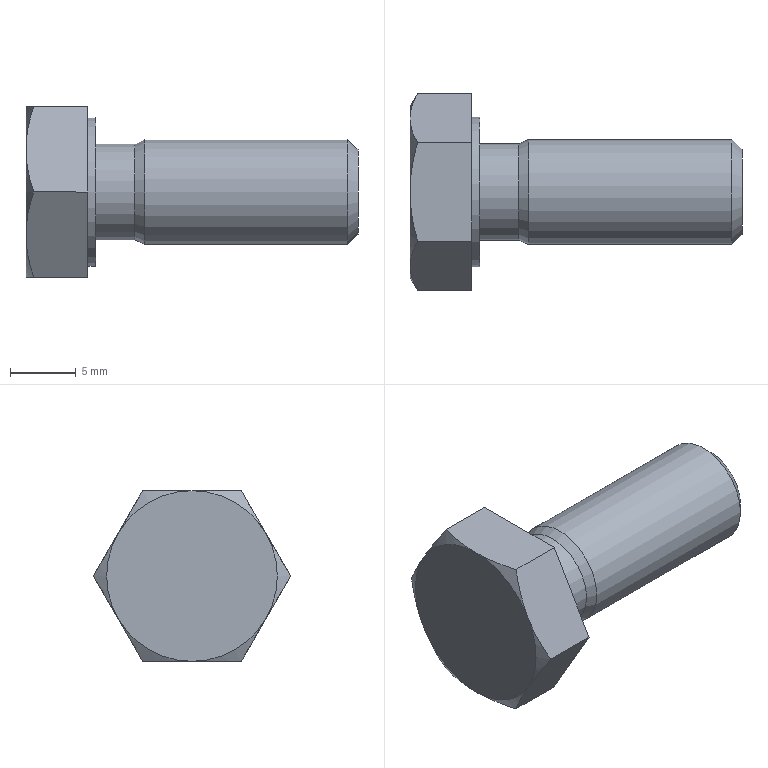Part | STEP file | DIN 933 - M8  x 20 | 1 solid | 21 faces | box 25.3 x 15.011 x 13 mm | volume 1718 mm3 | plane 10 | cone 8 | cylinder 3 | commonest cylinder face diameters 7.323 x1 8 x1 11.4 x1